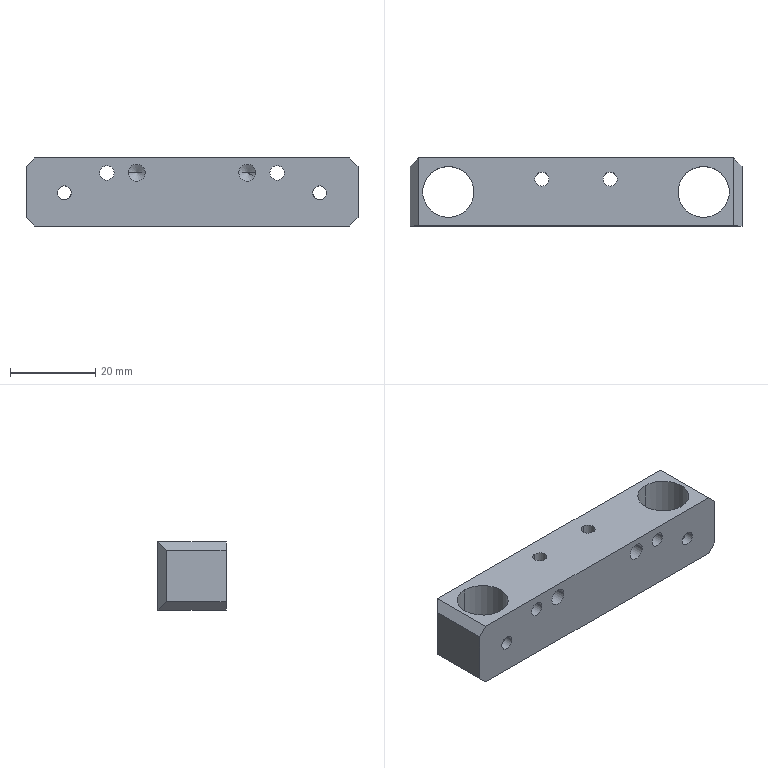NC program | NX | posted with a generic post | part box 78 x 16 x 16 mm
Lines 911 to 1853 of 3743:
(ZLEVEL_PROFILE , TOOL : D10)
N1802 T04 M6
N1804 G54
N1806 G17 G0 G90 X46.319 Y-8.34 B0. C0. S3500 M3
N1808 G43 Z30. H4
N1810 Z-0.219
N1812 G94 G1 X44.826 Y-7.944 F1000.
N1814 G3 X43.861 Y-8.205 R1.
N1816 G1 X42.573 Y-9.498 F2200.
N1818 X40.536 Y-11.536
N1820 X39.967 Y-12.025
N1822 X39.961 Y-12.104
N1824 X39.224 Y-12.843
N1826 G3 X38.966 Y-13.809 R1.
N1828 G1 X39.368 Y-15.302
N1830 G0 Z-0.438
N1832 G1 X38.966 Y-13.809 F1000.
N1834 G2 X39.224 Y-12.843 R1.
N1836 G1 X39.961 Y-12.104 F2200.
N1838 X39.967 Y-12.025
N1840 X40.536 Y-11.536
N1842 X42.573 Y-9.498
N1844 X43.861 Y-8.205
N1846 G2 X44.826 Y-7.944 R1.
N1848 G1 X46.319 Y-8.34
N1850 G0 Z-0.658
N1852 G1 X44.826 Y-7.944 F1000.
N1854 G3 X43.861 Y-8.205 R1.
N1856 G1 X42.573 Y-9.498 F2200.
N1858 X40.536 Y-11.536
N1860 X39.967 Y-12.025
N1862 X39.961 Y-12.104
N1864 X39.224 Y-12.843
N1866 G3 X38.966 Y-13.809 R1.
N1868 G1 X39.368 Y-15.302
N1870 G0 Z-0.877
N1872 G1 X38.966 Y-13.809 F1000.
N1874 G2 X39.224 Y-12.843 R1.
N1876 G1 X39.961 Y-12.104 F2200.
N1878 X39.967 Y-12.025
N1880 X40.536 Y-11.536
N1882 X42.573 Y-9.498
N1884 X43.861 Y-8.205
N1886 G2 X44.826 Y-7.944 R1.
N1888 G1 X46.319 Y-8.34
N1890 G0 Z-1.096
N1892 G1 X44.826 Y-7.944 F1000.
N1894 G3 X43.861 Y-8.205 R1.
N1896 G1 X42.573 Y-9.498 F2200.
N1898 X40.536 Y-11.536
N1900 X39.967 Y-12.025
N1902 X39.961 Y-12.104
N1904 X39.224 Y-12.843
N1906 G3 X38.966 Y-13.809 R1.
N1908 G1 X39.368 Y-15.302
N1910 G0 Z-1.315
N1912 G1 X38.966 Y-13.809 F1000.
N1914 G2 X39.224 Y-12.843 R1.
N1916 G1 X39.961 Y-12.104 F2200.
N1918 X39.967 Y-12.025
N1920 X40.536 Y-11.536
N1922 X42.573 Y-9.498
N1924 X43.861 Y-8.205
N1926 G2 X44.826 Y-7.944 R1.
N1928 G1 X46.319 Y-8.341
N1930 G0 Z-1.534
N1932 G1 X44.826 Y-7.944 F1000.
N1934 G3 X43.861 Y-8.205 R1.
N1936 G1 X42.573 Y-9.498 F2200.
N1938 X40.536 Y-11.536
N1940 X39.967 Y-12.025
N1942 X39.961 Y-12.104
N1944 X39.224 Y-12.843
N1946 G3 X38.966 Y-13.809 R1.
N1948 G1 X39.368 Y-15.302
N1950 G0 Z-1.753
N1952 G1 X38.966 Y-13.809 F1000.
N1954 G2 X39.224 Y-12.843 R1.
N1956 G1 X39.961 Y-12.104 F2200.
N1958 X39.967 Y-12.025
N1960 X40.536 Y-11.536
N1962 X42.573 Y-9.498
N1964 X43.861 Y-8.205
N1966 G2 X44.826 Y-7.944 R1.
N1968 G1 X46.319 Y-8.341
N1970 G0 Z-1.973
N1972 G1 X44.826 Y-7.944 F1000.
N1974 G3 X43.861 Y-8.205 R1.
N1976 G1 X42.573 Y-9.498 F2200.
N1978 X40.536 Y-11.536
N1980 X39.967 Y-12.025
N1982 X39.961 Y-12.104
N1984 X39.224 Y-12.843
N1986 G3 X38.966 Y-13.809 R1.
N1988 G1 X39.368 Y-15.302
N1990 G0 Z-2.192
N1992 G1 X38.966 Y-13.809 F1000.
N1994 G2 X39.224 Y-12.843 R1.
N1996 G1 X39.961 Y-12.104 F2200.
N1998 X39.967 Y-12.025
N2000 X40.536 Y-11.536
N2002 X42.573 Y-9.498
N2004 X43.861 Y-8.205
N2006 G2 X44.826 Y-7.944 R1.
N2008 G1 X46.319 Y-8.341
N2010 G0 Z-2.411
N2012 G1 X44.827 Y-7.944 F1000.
N2014 G3 X43.861 Y-8.205 R1.
N2016 G1 X42.573 Y-9.498 F2200.
N2018 X40.536 Y-11.536
N2020 X39.967 Y-12.025
N2022 X39.961 Y-12.104
N2024 X39.224 Y-12.843
N2026 G3 X38.966 Y-13.809 R1.
N2028 G1 X39.368 Y-15.303
N2030 G0 Z-2.63
N2032 G1 X38.966 Y-13.809 F1000.
N2034 G2 X39.224 Y-12.843 R1.
N2036 G1 X39.961 Y-12.104 F2200.
N2038 X39.967 Y-12.025
N2040 X40.536 Y-11.536
N2042 X42.573 Y-9.498
N2044 X43.861 Y-8.205
N2046 G2 X44.827 Y-7.944 R1.
N2048 G1 X46.319 Y-8.341
N2050 G0 Z-2.849
N2052 G1 X44.827 Y-7.944 F1000.
N2054 G3 X43.861 Y-8.205 R1.
N2056 G1 X42.573 Y-9.498 F2200.
N2058 X40.536 Y-11.536
N2060 X39.967 Y-12.025
N2062 X39.961 Y-12.104
N2064 X39.224 Y-12.843
N2066 G3 X38.966 Y-13.809 R1.
N2068 G1 X39.368 Y-15.303
N2070 G0 Z-3.068
N2072 G1 X38.966 Y-13.809 F1000.
N2074 G2 X39.224 Y-12.843 R1.
N2076 G1 X39.961 Y-12.104 F2200.
N2078 X39.967 Y-12.025
N2080 X40.536 Y-11.536
N2082 X42.573 Y-9.498
N2084 X43.861 Y-8.205
N2086 G2 X44.827 Y-7.945 R1.
N2088 G1 X46.319 Y-8.341
N2090 G0 Z-3.288
N2092 G1 X44.827 Y-7.945 F1000.
N2094 G3 X43.861 Y-8.205 R1.
N2096 G1 X42.573 Y-9.498 F2200.
N2098 X40.536 Y-11.536
N2100 X39.967 Y-12.025
N2102 X39.961 Y-12.105
N2104 X39.224 Y-12.843
N2106 G3 X38.966 Y-13.809 R1.
N2108 G1 X39.368 Y-15.303
N2110 G0 Z-3.507
N2112 G1 X38.966 Y-13.809 F1000.
N2114 G2 X39.224 Y-12.843 R1.
N2116 G1 X39.961 Y-12.105 F2200.
N2118 X39.967 Y-12.025
N2120 X40.536 Y-11.536
N2122 X42.573 Y-9.498
N2124 X43.861 Y-8.205
N2126 G2 X44.827 Y-7.945 R1.
N2128 G1 X46.319 Y-8.342
N2130 G0 Z-3.726
N2132 G1 X44.827 Y-7.945 F1000.
N2134 G3 X43.861 Y-8.205 R1.
N2136 G1 X42.573 Y-9.498 F2200.
N2138 X40.536 Y-11.536
N2140 X39.967 Y-12.025
N2142 X39.961 Y-12.105
N2144 X39.224 Y-12.843
N2146 G3 X38.966 Y-13.809 R1.
N2148 G1 X39.368 Y-15.303
N2150 G0 Z-3.945
N2152 G1 X38.966 Y-13.809 F1000.
N2154 G2 X39.224 Y-12.843 R1.
N2156 G1 X39.961 Y-12.105 F2200.
N2158 X39.967 Y-12.025
N2160 X40.536 Y-11.536
N2162 X42.573 Y-9.498
N2164 X43.861 Y-8.205
N2166 G2 X44.827 Y-7.945 R1.
N2168 G1 X46.319 Y-8.342
N2170 G0 Z-4.164
N2172 G1 X44.827 Y-7.945 F1000.
N2174 G3 X43.861 Y-8.205 R1.
N2176 G1 X42.573 Y-9.498 F2200.
N2178 X40.536 Y-11.536
N2180 X39.967 Y-12.025
N2182 X39.962 Y-12.105
N2184 X39.224 Y-12.843
N2186 G3 X38.966 Y-13.809 R1.
N2188 G1 X39.368 Y-15.303
N2190 G0 Z-4.384
N2192 G1 X38.966 Y-13.809 F1000.
N2194 G2 X39.224 Y-12.843 R1.
N2196 G1 X39.962 Y-12.105 F2200.
N2198 X39.967 Y-12.025
N2200 X40.536 Y-11.536
N2202 X42.573 Y-9.498
N2204 X43.861 Y-8.205
N2206 G2 X44.827 Y-7.945 R1.
N2208 G1 X46.319 Y-8.342
N2210 G0 Z-4.603
N2212 G1 X44.827 Y-7.945 F1000.
N2214 G3 X43.861 Y-8.205 R1.
N2216 G1 X42.573 Y-9.498 F2200.
N2218 X40.536 Y-11.536
N2220 X39.967 Y-12.025
N2222 X39.962 Y-12.105
N2224 X39.224 Y-12.843
N2226 G3 X38.966 Y-13.809 R1.
N2228 G1 X39.368 Y-15.303
N2230 G0 Z-4.822
N2232 G1 X38.966 Y-13.809 F1000.
N2234 G2 X39.224 Y-12.843 R1.
N2236 G1 X39.962 Y-12.105 F2200.
N2238 X39.967 Y-12.025
N2240 X40.536 Y-11.536
N2242 X42.573 Y-9.498
N2244 X43.862 Y-8.205
N2246 G2 X44.827 Y-7.945 R1.
N2248 G1 X46.319 Y-8.342
N2250 G0 Z-5.041
N2252 G1 X44.827 Y-7.945 F1000.
N2254 G3 X43.862 Y-8.205 R1.
N2256 G1 X42.573 Y-9.498 F2200.
N2258 X40.536 Y-11.536
N2260 X39.967 Y-12.025
N2262 X39.962 Y-12.105
N2264 X39.224 Y-12.843
N2266 G3 X38.966 Y-13.81 R1.
N2268 G1 X39.368 Y-15.303
N2270 G0 Z-5.26
N2272 G1 X38.966 Y-13.81 F1000.
N2274 G2 X39.224 Y-12.843 R1.
N2276 G1 X39.962 Y-12.105 F2200.
N2278 X39.967 Y-12.025
N2280 X40.536 Y-11.536
N2282 X42.573 Y-9.498
N2284 X43.862 Y-8.205
N2286 G2 X44.827 Y-7.945 R1.
N2288 G1 X46.319 Y-8.342
N2290 G0 Y-8.343 Z-5.479
N2292 G1 X44.827 Y-7.945 F1000.
N2294 G3 X43.862 Y-8.206 R1.
N2296 G1 X42.573 Y-9.498 F2200.
N2298 X40.536 Y-11.536
N2300 X39.967 Y-12.025
N2302 X39.962 Y-12.105
N2304 X39.224 Y-12.843
N2306 G3 X38.967 Y-13.81 R1.
N2308 G1 X39.368 Y-15.303
N2310 G0 Z-5.699
N2312 G1 X38.967 Y-13.81 F1000.
N2314 G2 X39.225 Y-12.843 R1.
N2316 G1 X39.962 Y-12.105 F2200.
N2318 X39.967 Y-12.025
N2320 X40.536 Y-11.536
N2322 X42.573 Y-9.498
N2324 X43.862 Y-8.206
N2326 G2 X44.827 Y-7.945 R1.
N2328 G1 X46.319 Y-8.343
N2330 G0 Z-5.918
N2332 G1 X44.827 Y-7.945 F1000.
N2334 G3 X43.862 Y-8.206 R1.
N2336 G1 X42.573 Y-9.498 F2200.
N2338 X40.536 Y-11.536
N2340 X39.967 Y-12.025
N2342 X39.962 Y-12.105
N2344 X39.225 Y-12.843
N2346 G3 X38.967 Y-13.81 R1.
N2348 G1 X39.368 Y-15.303
N2350 G0 Z-6.137
N2352 G1 X38.967 Y-13.81 F1000.
N2354 G2 X39.225 Y-12.844 R1.
N2356 G1 X39.962 Y-12.105 F2200.
N2358 X39.967 Y-12.025
N2360 X40.536 Y-11.536
N2362 X42.573 Y-9.498
N2364 X43.862 Y-8.206
N2366 G2 X44.827 Y-7.945 R1.
N2368 G1 X46.319 Y-8.343
N2370 G0 Z-6.356
N2372 G1 X44.827 Y-7.946 F1000.
N2374 G3 X43.862 Y-8.206 R1.
N2376 G1 X42.573 Y-9.498 F2200.
N2378 X40.536 Y-11.536
N2380 X39.967 Y-12.025
N2382 X39.962 Y-12.105
N2384 X39.225 Y-12.844
N2386 G3 X38.967 Y-13.81 R1.
N2388 G1 X39.368 Y-15.303
N2390 G0 Z-6.575
N2392 G1 X38.967 Y-13.81 F1000.
N2394 G2 X39.225 Y-12.844 R1.
N2396 G1 X39.962 Y-12.105 F2200.
N2398 X39.967 Y-12.025
N2400 X40.536 Y-11.536
N2402 X42.573 Y-9.498
N2404 X43.862 Y-8.206
N2406 G2 X44.827 Y-7.946 R1.
N2408 G1 X46.319 Y-8.343
N2410 G0 Z-6.795
N2412 G1 X44.827 Y-7.946 F1000.
N2414 G3 X43.862 Y-8.206 R1.
N2416 G1 X42.573 Y-9.498 F2200.
N2418 X40.536 Y-11.536
N2420 X39.967 Y-12.025
N2422 X39.962 Y-12.105
N2424 X39.225 Y-12.844
N2426 G3 X38.967 Y-13.81 R1.
N2428 G1 X39.368 Y-15.303
N2430 G0 Z-7.014
N2432 G1 X38.967 Y-13.81 F1000.
N2434 G2 X39.225 Y-12.844 R1.
N2436 G1 X39.962 Y-12.105 F2200.
N2438 X39.967 Y-12.025
N2440 X40.536 Y-11.536
N2442 X42.573 Y-9.498
N2444 X43.862 Y-8.206
N2446 G2 X44.828 Y-7.946 R1.
N2448 G1 X46.319 Y-8.343
N2450 G0 Z-7.233
N2452 G1 X44.828 Y-7.946 F1000.
N2454 G3 X43.862 Y-8.206 R1.
N2456 G1 X42.573 Y-9.498 F2200.
N2458 X40.536 Y-11.536
N2460 X39.967 Y-12.025
N2462 X39.962 Y-12.105
N2464 X39.225 Y-12.844
N2466 G3 X38.967 Y-13.81 R1.
N2468 G1 X39.368 Y-15.303
N2470 G0 Z-7.452
N2472 G1 X38.967 Y-13.81 F1000.
N2474 G2 X39.225 Y-12.844 R1.
N2476 G1 X39.962 Y-12.105 F2200.
N2478 X39.967 Y-12.025
N2480 X40.536 Y-11.536
N2482 X42.573 Y-9.498
N2484 X43.862 Y-8.206
N2486 G2 X44.828 Y-7.946 R1.
N2488 G1 X46.319 Y-8.343
N2490 G0 Y-8.344 Z-7.671
N2492 G1 X44.828 Y-7.946 F1000.
N2494 G3 X43.862 Y-8.206 R1.
N2496 G1 X42.573 Y-9.498 F2200.
N2498 X40.536 Y-11.536
N2500 X39.967 Y-12.025
N2502 X39.962 Y-12.105
N2504 X39.225 Y-12.844
N2506 G3 X38.967 Y-13.81 R1.
N2508 G1 X39.368 Y-15.303
N2510 G0 Y-15.304 Z-7.89
N2512 G1 X38.967 Y-13.81 F1000.
N2514 G2 X39.225 Y-12.844 R1.
N2516 G1 X39.962 Y-12.105 F2200.
N2518 X39.967 Y-12.025
N2520 X40.536 Y-11.536
N2522 X42.573 Y-9.498
N2524 X43.862 Y-8.206
N2526 G2 X44.828 Y-7.946 R1.
N2528 G1 X46.319 Y-8.344
N2530 G0 Z-8.11
N2532 G1 X44.828 Y-7.946 F1000.
N2534 G3 X43.862 Y-8.206 R1.
N2536 G1 X42.573 Y-9.498 F2200.
N2538 X40.536 Y-11.536
N2540 X39.967 Y-12.025
N2542 X39.962 Y-12.105
N2544 X39.225 Y-12.844
N2546 G3 X38.967 Y-13.81 R1.
N2548 G1 X39.368 Y-15.304
N2550 G0 Z-8.329
N2552 G1 X38.967 Y-13.81 F1000.
N2554 G2 X39.225 Y-12.844 R1.
N2556 G1 X39.962 Y-12.105 F2200.
N2558 X39.967 Y-12.025
N2560 X40.536 Y-11.536
N2562 X42.573 Y-9.498
N2564 X43.862 Y-8.206
N2566 G2 X44.828 Y-7.946 R1.
N2568 G1 X46.319 Y-8.344
N2570 G0 Z-8.548
N2572 G1 X44.828 Y-7.946 F1000.
N2574 G3 X43.862 Y-8.206 R1.
N2576 G1 X42.573 Y-9.498 F2200.
N2578 X40.536 Y-11.536
N2580 X39.967 Y-12.025
N2582 X39.962 Y-12.105
N2584 X39.225 Y-12.844
N2586 G3 X38.967 Y-13.81 R1.
N2588 G1 X39.368 Y-15.304
N2590 G0 Z-8.767
N2592 G1 X38.967 Y-13.81 F1000.
N2594 G2 X39.225 Y-12.844 R1.
N2596 G1 X39.962 Y-12.105 F2200.
N2598 X39.967 Y-12.025
N2600 X40.536 Y-11.536
N2602 X42.573 Y-9.498
N2604 X43.862 Y-8.206
N2606 G2 X44.828 Y-7.946 R1.
N2608 G1 X46.319 Y-8.344
N2610 G0 Z-8.986
N2612 G1 X44.828 Y-7.946 F1000.
N2614 G3 X43.862 Y-8.206 R1.
N2616 G1 X42.573 Y-9.498 F2200.
N2618 X40.536 Y-11.536
N2620 X39.967 Y-12.025
N2622 X39.962 Y-12.105
N2624 X39.225 Y-12.844
N2626 G3 X38.967 Y-13.81 R1.
N2628 G1 X39.368 Y-15.304
N2630 G0 Z-9.205
N2632 G1 X38.967 Y-13.81 F1000.
N2634 G2 X39.225 Y-12.844 R1.
N2636 G1 X39.962 Y-12.105 F2200.
N2638 X39.967 Y-12.025
N2640 X40.536 Y-11.536
N2642 X42.573 Y-9.498
N2644 X43.862 Y-8.206
N2646 G2 X44.828 Y-7.946 R1.
N2648 G1 X46.319 Y-8.344
N2650 G0 Z-9.425
N2652 G1 X44.828 Y-7.946 F1000.
N2654 G3 X43.862 Y-8.206 R1.
N2656 G1 X42.573 Y-9.498 F2200.
N2658 X40.536 Y-11.536
N2660 X39.967 Y-12.025
N2662 X39.962 Y-12.105
N2664 X39.225 Y-12.844
N2666 G3 X38.967 Y-13.81 R1.
N2668 G1 X39.369 Y-15.304
N2670 G0 Z-9.644
N2672 G1 X38.967 Y-13.81 F1000.
N2674 G2 X39.225 Y-12.844 R1.
N2676 G1 X39.962 Y-12.105 F2200.
N2678 X39.967 Y-12.025
N2680 X40.536 Y-11.536
N2682 X42.573 Y-9.498
N2684 X43.862 Y-8.206
N2686 G2 X44.828 Y-7.947 R1.
N2688 G1 X46.319 Y-8.344
N2690 G0 Y-8.345 Z-9.863
N2692 G1 X44.828 Y-7.947 F1000.
N2694 G3 X43.862 Y-8.206 R1.
N2696 G1 X42.573 Y-9.498 F2200.
N2698 X40.536 Y-11.536
N2700 X39.967 Y-12.025
N2702 X39.962 Y-12.106
N2704 X39.225 Y-12.844
N2706 G3 X38.967 Y-13.81 R1.
N2708 G1 X39.369 Y-15.304
N2710 G0 Z-10.082
N2712 G1 X38.967 Y-13.81 F1000.
N2714 G2 X39.225 Y-12.844 R1.
N2716 G1 X39.962 Y-12.106 F2200.
N2718 X39.967 Y-12.025
N2720 X40.536 Y-11.536
N2722 X42.573 Y-9.498
N2724 X43.862 Y-8.206
N2726 G2 X44.828 Y-7.947 R1.
N2728 G1 X46.319 Y-8.345
N2730 G0 Z-10.301
N2732 G1 X44.828 Y-7.947 F1000.
N2734 G3 X43.863 Y-8.206 R1.
N2736 G1 X42.573 Y-9.498 F2200.
N2738 X40.536 Y-11.536
N2740 X39.967 Y-12.025
N2742 X39.962 Y-12.106
N2744 X39.225 Y-12.844
N2746 G3 X38.967 Y-13.81 R1.
N2748 G1 X39.369 Y-15.304
N2750 G0 Z-10.521
N2752 G1 X38.967 Y-13.81 F1000.
N2754 G2 X39.225 Y-12.844 R1.
N2756 G1 X39.963 Y-12.106 F2200.
N2758 X39.967 Y-12.025
N2760 X40.536 Y-11.536
N2762 X42.573 Y-9.498
N2764 X43.863 Y-8.206
N2766 G2 X44.828 Y-7.947 R1.
N2768 G1 X46.319 Y-8.345
N2770 G0 X46.318 Z-10.74
N2772 G1 X44.828 Y-7.947 F1000.
N2774 G3 X43.863 Y-8.206 R1.
N2776 G1 X42.573 Y-9.498 F2200.
N2778 X40.536 Y-11.536
N2780 X39.967 Y-12.025
N2782 X39.963 Y-12.106
N2784 X39.225 Y-12.844
N2786 G3 X38.967 Y-13.81 R1.
N2788 G1 X39.369 Y-15.304
N2790 G0 Z-10.959
N2792 G1 X38.967 Y-13.81 F1000.
N2794 G2 X39.225 Y-12.844 R1.
N2796 G1 X39.963 Y-12.106 F2200.
N2798 X39.967 Y-12.025
N2800 X40.536 Y-11.536
N2802 X42.573 Y-9.498
N2804 X43.863 Y-8.206
N2806 G2 X44.828 Y-7.947 R1.
N2808 G1 X46.318 Y-8.345
N2810 G0 Z-11.178
N2812 G1 X44.828 Y-7.947 F1000.
N2814 G3 X43.863 Y-8.207 R1.
N2816 G1 X42.573 Y-9.498 F2200.
N2818 X40.536 Y-11.536
N2820 X39.967 Y-12.025
N2822 X39.963 Y-12.106
N2824 X39.225 Y-12.844
N2826 G3 X38.967 Y-13.81 R1.
N2828 G1 X39.369 Y-15.304
N2830 G0 Z-11.397
N2832 G1 X38.967 Y-13.81 F1000.
N2834 G2 X39.225 Y-12.844 R1.
N2836 G1 X39.963 Y-12.106 F2200.
N2838 X39.967 Y-12.025
N2840 X40.536 Y-11.536
N2842 X42.573 Y-9.498
N2844 X43.863 Y-8.207
N2846 G2 X44.828 Y-7.947 R1.
N2848 G1 X46.318 Y-8.345
N2850 G0 Z-11.616
N2852 G1 X44.829 Y-7.947 F1000.
N2854 G3 X43.863 Y-8.207 R1.
N2856 G1 X42.573 Y-9.498 F2200.
N2858 X40.536 Y-11.536
N2860 X39.967 Y-12.025
N2862 X39.963 Y-12.106
N2864 X39.225 Y-12.844
N2866 G3 X38.967 Y-13.81 R1.
N2868 G1 X39.369 Y-15.304
N2870 G0 Z-11.836
N2872 G1 X38.967 Y-13.81 F1000.
N2874 G2 X39.225 Y-12.844 R1.
N2876 G1 X39.963 Y-12.106 F2200.
N2878 X39.967 Y-12.025
N2880 X40.536 Y-11.536
N2882 X42.573 Y-9.498
N2884 X43.863 Y-8.207
N2886 G2 X44.829 Y-7.947 R1.
N2888 G1 X46.318 Y-8.345
N2890 G0 Z-12.055
N2892 G1 X44.829 Y-7.947 F1000.
N2894 G3 X43.863 Y-8.207 R1.
N2896 G1 X42.573 Y-9.498 F2200.
N2898 X40.536 Y-11.536
N2900 X39.967 Y-12.025
N2902 X39.963 Y-12.106
N2904 X39.225 Y-12.844
N2906 G3 X38.967 Y-13.81 R1.
N2908 G1 X39.369 Y-15.304
N2910 G0 Z-12.274
N2912 G1 X38.967 Y-13.811 F1000.
N2914 G2 X39.225 Y-12.844 R1.
N2916 G1 X39.963 Y-12.106 F2200.
N2918 X39.967 Y-12.025
N2920 X40.536 Y-11.536
N2922 X42.573 Y-9.498
N2924 X43.863 Y-8.207
N2926 G2 X44.829 Y-7.947 R1.
N2928 G1 X46.318 Y-8.346
N2930 G0 Z-12.493
N2932 G1 X44.829 Y-7.947 F1000.
N2934 G3 X43.863 Y-8.207 R1.
N2936 G1 X42.573 Y-9.498 F2200.
N2938 X40.536 Y-11.536
N2940 X39.967 Y-12.025
N2942 X39.963 Y-12.106
N2944 X39.225 Y-12.844
N2946 G3 X38.967 Y-13.811 R1.
N2948 G1 X39.369 Y-15.304
N2950 G0 Z-12.712
N2952 G1 X38.967 Y-13.811 F1000.
N2954 G2 X39.225 Y-12.844 R1.
N2956 G1 X39.963 Y-12.106 F2200.
N2958 X39.967 Y-12.025
N2960 X40.536 Y-11.536
N2962 X42.573 Y-9.498
N2964 X43.863 Y-8.207
N2966 G2 X44.829 Y-7.947 R1.
N2968 G1 X46.318 Y-8.346
N2970 G0 Z-12.932
N2972 G1 X44.829 Y-7.948 F1000.
N2974 G3 X43.863 Y-8.207 R1.
N2976 G1 X42.573 Y-9.498 F2200.
N2978 X40.536 Y-11.536
N2980 X39.967 Y-12.025
N2982 X39.963 Y-12.106
N2984 X39.225 Y-12.844
N2986 G3 X38.967 Y-13.811 R1.
N2988 G1 X39.369 Y-15.304
N2990 G0 Z-13.151
N2992 G1 X38.967 Y-13.811 F1000.
N2994 G2 X39.226 Y-12.845 R1.
N2996 G1 X39.963 Y-12.106 F2200.
N2998 X39.967 Y-12.025
N3000 X40.536 Y-11.536
N3002 X42.573 Y-9.498
N3004 X43.863 Y-8.207
N3006 G2 X44.829 Y-7.948 R1.
N3008 G1 X46.318 Y-8.346
N3010 G0 Z-13.37
N3012 G1 X44.829 Y-7.948 F1000.
N3014 G3 X43.863 Y-8.207 R1.
N3016 G1 X42.573 Y-9.498 F2200.
N3018 X40.536 Y-11.536
N3020 X39.967 Y-12.025
N3022 X39.963 Y-12.106
N3024 X39.226 Y-12.845
N3026 G3 X38.967 Y-13.811 R1.
N3028 G1 X39.369 Y-15.305
N3030 G0 Z-13.589
N3032 G1 X38.967 Y-13.811 F1000.
N3034 G2 X39.226 Y-12.845 R1.
N3036 G1 X39.963 Y-12.106 F2200.
N3038 X39.967 Y-12.025
N3040 X40.536 Y-11.536
N3042 X42.573 Y-9.498
N3044 X43.863 Y-8.207
N3046 G2 X44.829 Y-7.948 R1.
N3048 G1 X46.318 Y-8.346
N3050 G0 Z-13.808
N3052 G1 X44.829 Y-7.948 F1000.
N3054 G3 X43.863 Y-8.207 R1.
N3056 G1 X42.573 Y-9.498 F2200.
N3058 X40.536 Y-11.536
N3060 X39.967 Y-12.025
N3062 X39.963 Y-12.106
N3064 X39.226 Y-12.845
N3066 G3 X38.967 Y-13.811 R1.
N3068 G1 X39.369 Y-15.305
N3070 G0 Z-14.027
N3072 G1 X38.968 Y-13.811 F1000.
N3074 G2 X39.226 Y-12.845 R1.
N3076 G1 X39.963 Y-12.106 F2200.
N3078 X39.967 Y-12.025
N3080 X40.536 Y-11.536
N3082 X42.508 Y-9.563
N3084 X43.863 Y-8.207
N3086 G2 X44.829 Y-7.948 R1.
N3088 G1 X46.318 Y-8.346
N3090 G0 Z-14.247
N3092 G1 X44.829 Y-7.948 F1000.
N3094 G3 X43.863 Y-8.207 R1.
N3096 G1 X42.508 Y-9.563 F2200.
N3098 X40.536 Y-11.536
N3100 X39.967 Y-12.025
N3102 X39.963 Y-12.106
N3104 X39.226 Y-12.845
N3106 G3 X38.968 Y-13.811 R1.
N3108 G1 X39.369 Y-15.305
N3110 G0 Z-14.466
N3112 G1 X38.968 Y-13.811 F1000.
N3114 G2 X39.226 Y-12.845 R1.
N3116 G1 X39.963 Y-12.106 F2200.
N3118 X39.967 Y-12.025
N3120 X40.536 Y-11.536
N3122 X42.508 Y-9.563
N3124 X43.863 Y-8.207
N3126 G2 X44.829 Y-7.948 R1.
N3128 G1 X46.318 Y-8.347
N3130 G0 Z-14.685
N3132 G1 X44.829 Y-7.948 F1000.
N3134 G3 X43.863 Y-8.207 R1.
N3136 G1 X42.508 Y-9.563 F2200.
N3138 X40.536 Y-11.536
N3140 X39.967 Y-12.025
N3142 X39.963 Y-12.106
N3144 X39.226 Y-12.845
N3146 G3 X38.968 Y-13.811 R1.
N3148 G1 X39.369 Y-15.305
N3150 G0 Z-14.904
N3152 G1 X38.968 Y-13.811 F1000.
N3154 G2 X39.226 Y-12.845 R1.
N3156 G1 X39.963 Y-12.106 F2200.
N3158 X39.967 Y-12.025
N3160 X40.536 Y-11.536
N3162 X42.508 Y-9.563
N3164 X43.863 Y-8.207
N3166 G2 X44.829 Y-7.948 R1.
N3168 G1 X46.318 Y-8.347
N3170 G0 Z-15.123
N3172 G1 X44.829 Y-7.948 F1000.
N3174 G3 X43.863 Y-8.207 R1.
N3176 G1 X42.508 Y-9.563 F2200.
N3178 X40.536 Y-11.536
N3180 X39.967 Y-12.025
N3182 X39.963 Y-12.106
N3184 X39.226 Y-12.845
N3186 G3 X38.968 Y-13.811 R1.
N3188 G1 X39.369 Y-15.305
N3190 G0 Z-15.342
N3192 G1 X38.968 Y-13.811 F1000.
N3194 G2 X39.226 Y-12.845 R1.
N3196 G1 X39.963 Y-12.106 F2200.
N3198 X39.967 Y-12.025
N3200 X40.536 Y-11.536
N3202 X42.508 Y-9.563
N3204 X43.863 Y-8.207
N3206 G2 X44.829 Y-7.948 R1.
N3208 G1 X46.318 Y-8.347
N3210 G0 Z-15.562
N3212 G1 X44.829 Y-7.948 F1000.
N3214 G3 X43.863 Y-8.207 R1.
N3216 G1 X42.508 Y-9.563 F2200.
N3218 X40.536 Y-11.536
N3220 X39.967 Y-12.025
N3222 X39.963 Y-12.106
N3224 X39.226 Y-12.845
N3226 G3 X38.968 Y-13.811 R1.
N3228 G1 X39.369 Y-15.305
N3230 G0 Z-15.781
N3232 G1 X38.968 Y-13.811 F1000.
N3234 G2 X39.226 Y-12.845 R1.
N3236 G1 X39.963 Y-12.106 F2200.
N3238 X39.967 Y-12.025
N3240 X40.536 Y-11.536
N3242 X42.508 Y-9.563
N3244 X43.863 Y-8.207
N3246 G2 X44.829 Y-7.948 R1.
N3248 G1 X46.318 Y-8.347
N3250 G0 Z-16.
N3252 G1 X44.829 Y-7.948 F1000.
N3254 G3 X43.863 Y-8.207 R1.
N3256 G1 X42.508 Y-9.563 F2200.
N3258 X40.536 Y-11.536
N3260 X39.967 Y-12.025
N3262 X39.963 Y-12.106
N3264 X39.226 Y-12.845
N3266 G3 X38.968 Y-13.811 R1.
N3268 G1 X39.369 Y-15.305
N3270 G0 Z30.
N3272 X39.365 Y15.303
N3274 Z-0.219
N3276 G1 X38.965 Y13.809 F1000.
N3278 G3 X39.224 Y12.843 R1.
N3280 G1 X41.067 Y11. F2200.
N3282 X41.251 Y10.82
N3284 X42.536 Y9.536
N3286 X42.609 Y9.457
N3288 X43.861 Y8.205
N3290 G3 X44.826 Y7.945 R1.
N3292 G1 X46.316 Y8.344
N3294 G0 Z-0.438
N3296 G1 X44.827 Y7.945 F1000.
N3298 G2 X43.861 Y8.205 R1.
N3300 G1 X42.609 Y9.457 F2200.
N3302 X42.536 Y9.536
N3304 X41.251 Y10.82
N3306 X41.067 Y11.
N3308 X39.224 Y12.843
N3310 G2 X38.965 Y13.809 R1.
N3312 G1 X39.365 Y15.303
N3314 G0 Z-0.658
N3316 G1 X38.965 Y13.809 F1000.
N3318 G3 X39.224 Y12.843 R1.
N3320 G1 X41.067 Y11. F2200.
N3322 X41.251 Y10.82
N3324 X42.536 Y9.536
N3326 X42.609 Y9.457
N3328 X43.861 Y8.205
N3330 G3 X44.827 Y7.945 R1.
N3332 G1 X46.316 Y8.344
N3334 G0 Z-0.877
N3336 G1 X44.827 Y7.945 F1000.
N3338 G2 X43.861 Y8.205 R1.
N3340 G1 X42.609 Y9.457 F2200.
N3342 X42.536 Y9.536
N3344 X41.251 Y10.82
N3346 X41.067 Y11.
N3348 X39.224 Y12.843
N3350 G2 X38.965 Y13.809 R1.
N3352 G1 X39.365 Y15.303
N3354 G0 Z-1.096
N3356 G1 X38.965 Y13.809 F1000.
N3358 G3 X39.224 Y12.843 R1.
N3360 G1 X41.067 Y11. F2200.
N3362 X41.251 Y10.82
N3364 X42.536 Y9.536
N3366 X42.609 Y9.457
N3368 X43.861 Y8.205
N3370 G3 X44.827 Y7.946 R1.
N3372 G1 X46.316 Y8.344
N3374 G0 Z-1.315
N3376 G1 X44.827 Y7.946 F1000.
N3378 G2 X43.861 Y8.205 R1.
N3380 G1 X42.609 Y9.457 F2200.
N3382 X42.536 Y9.536
N3384 X41.251 Y10.82
N3386 X41.067 Y11.
N3388 X39.224 Y12.843
N3390 G2 X38.965 Y13.809 R1.
N3392 G1 X39.365 Y15.303
N3394 G0 Z-1.534
N3396 G1 X38.965 Y13.809 F1000.
N3398 G3 X39.224 Y12.843 R1.
N3400 G1 X41.067 Y11. F2200.
N3402 X41.251 Y10.82
N3404 X42.536 Y9.536
N3406 X42.609 Y9.457
N3408 X43.861 Y8.205
N3410 G3 X44.827 Y7.946 R1.
N3412 G1 X46.317 Y8.344
N3414 G0 Z-1.753
N3416 G1 X44.827 Y7.946 F1000.
N3418 G2 X43.861 Y8.205 R1.
N3420 G1 X42.609 Y9.457 F2200.
N3422 X42.536 Y9.536
N3424 X41.251 Y10.82
N3426 X41.067 Y11.
N3428 X39.224 Y12.843
N3430 G2 X38.965 Y13.809 R1.
N3432 G1 X39.365 Y15.303
N3434 G0 Z-1.973
N3436 G1 X38.965 Y13.809 F1000.
N3438 G3 X39.224 Y12.843 R1.
N3440 G1 X41.067 Y11. F2200.
N3442 X41.251 Y10.82
N3444 X42.536 Y9.536
N3446 X42.609 Y9.458
N3448 X43.861 Y8.205
N3450 G3 X44.827 Y7.946 R1.
N3452 G1 X46.317 Y8.344
N3454 G0 Z-2.192
N3456 G1 X44.827 Y7.946 F1000.
N3458 G2 X43.861 Y8.205 R1.
N3460 G1 X42.609 Y9.458 F2200.
N3462 X42.536 Y9.536
N3464 X41.251 Y10.82
N3466 X41.067 Y11.
N3468 X39.224 Y12.843
N3470 G2 X38.965 Y13.809 R1.
N3472 G1 X39.365 Y15.304
N3474 G0 Z-2.411
N3476 G1 X38.965 Y13.809 F1000.
N3478 G3 X39.224 Y12.843 R1.
N3480 G1 X41.067 Y11. F2200.
N3482 X41.251 Y10.82
N3484 X42.536 Y9.536
N3486 X42.609 Y9.458
N3488 X43.861 Y8.205
N3490 G3 X44.827 Y7.946 R1.
N3492 G1 X46.317 Y8.344
N3494 G0 Z-2.63
N3496 G1 X44.827 Y7.946 F1000.
N3498 G2 X43.861 Y8.205 R1.
N3500 G1 X42.609 Y9.458 F2200.
N3502 X42.536 Y9.536
N3504 X41.251 Y10.82
N3506 X41.067 Y11.
N3508 X39.224 Y12.843
N3510 G2 X38.965 Y13.809 R1.
N3512 G1 X39.365 Y15.304
N3514 G0 Z-2.849
N3516 G1 X38.965 Y13.809 F1000.
N3518 G3 X39.224 Y12.843 R1.
N3520 G1 X41.067 Y11. F2200.
N3522 X41.251 Y10.82
N3524 X42.536 Y9.536
N3526 X42.609 Y9.458
N3528 X43.861 Y8.205
N3530 G3 X44.827 Y7.946 R1.
N3532 G1 X46.317 Y8.344
N3534 G0 Y8.345 Z-3.068
N3536 G1 X44.827 Y7.946 F1000.
N3538 G2 X43.861 Y8.205 R1.
N3540 G1 X42.609 Y9.458 F2200.
N3542 X42.536 Y9.536
N3544 X41.251 Y10.82
N3546 X41.067 Y11.
N3548 X39.224 Y12.843
N3550 G2 X38.965 Y13.809 R1.
N3552 G1 X39.365 Y15.304
N3554 G0 X39.366 Z-3.288
N3556 G1 X38.965 Y13.809 F1000.
N3558 G3 X39.224 Y12.843 R1.
N3560 G1 X41.067 Y11. F2200.
N3562 X41.251 Y10.82
N3564 X42.536 Y9.536
N3566 X42.609 Y9.458
N3568 X43.861 Y8.205
N3570 G3 X44.827 Y7.946 R1.
N3572 G1 X46.317 Y8.345
N3574 G0 Z-3.507
N3576 G1 X44.827 Y7.946 F1000.
N3578 G2 X43.861 Y8.205 R1.
N3580 G1 X42.609 Y9.458 F2200.
N3582 X42.536 Y9.536
N3584 X41.251 Y10.82
N3586 X41.067 Y11.001
N3588 X39.224 Y12.843
N3590 G2 X38.965 Y13.809 R1.
N3592 G1 X39.366 Y15.304
N3594 G0 Z-3.726
N3596 G1 X38.965 Y13.809 F1000.
N3598 G3 X39.224 Y12.843 R1.
N3600 G1 X41.067 Y11.001 F2200.
N3602 X41.251 Y10.82
N3604 X42.536 Y9.536
N3606 X42.609 Y9.458
N3608 X43.861 Y8.205
N3610 G3 X44.827 Y7.946 R1.
N3612 G1 X46.317 Y8.345
N3614 G0 Z-3.945
N3616 G1 X44.827 Y7.946 F1000.
N3618 G2 X43.861 Y8.205 R1.
N3620 G1 X42.609 Y9.458 F2200.
N3622 X42.536 Y9.536
N3624 X41.251 Y10.82
N3626 X41.067 Y11.001
N3628 X39.224 Y12.843
N3630 G2 X38.965 Y13.809 R1.
N3632 G1 X39.366 Y15.304
N3634 G0 Z-4.164
N3636 G1 X38.965 Y13.809 F1000.
N3638 G3 X39.224 Y12.843 R1.
N3640 G1 X41.067 Y11.001 F2200.
N3642 X41.251 Y10.82
N3644 X42.536 Y9.536
N3646 X42.609 Y9.458
N3648 X43.861 Y8.205
N3650 G3 X44.827 Y7.946 R1.
N3652 G1 X46.317 Y8.345
N3654 G0 Z-4.384
N3656 G1 X44.827 Y7.946 F1000.
N3658 G2 X43.861 Y8.205 R1.
N3660 G1 X42.609 Y9.458 F2200.
N3662 X42.536 Y9.536
N3664 X41.251 Y10.82
N3666 X41.067 Y11.001
N3668 X39.224 Y12.843
N3670 G2 X38.965 Y13.809 R1.
N3672 G1 X39.366 Y15.304
N3674 G0 Z-4.603
N3676 G1 X38.965 Y13.809 F1000.
N3678 G3 X39.224 Y12.843 R1.
N3680 G1 X41.067 Y11.001 F2200.